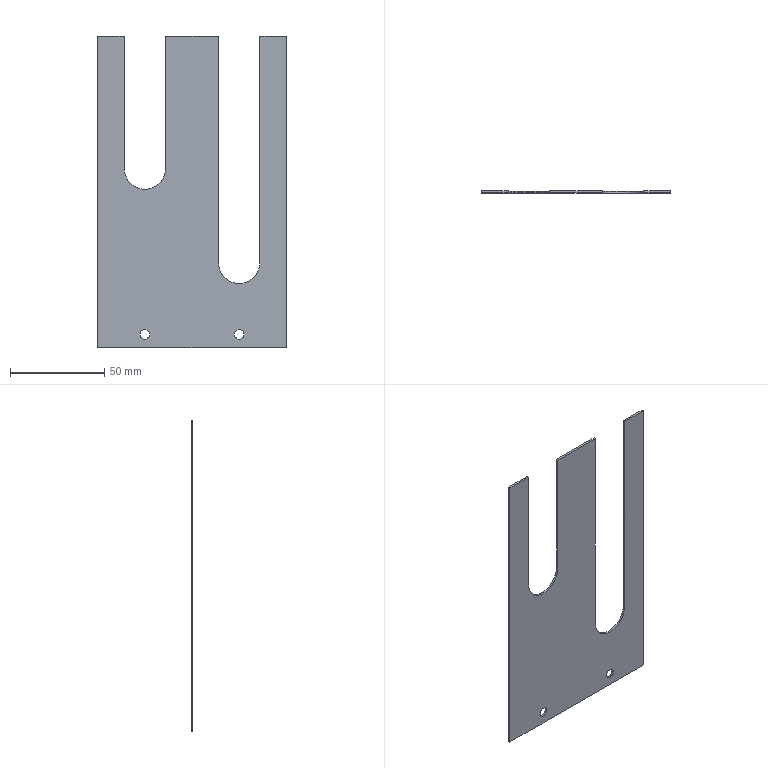Part | SolidWorks | features Extrusion 1, ICE 1 | 1 solid | 18 faces | box 100 x 1 x 165 mm | volume 11901 mm3 | plane 12 | cylinder 6 | commonest cylinder face diameters 5 x4 22 x2
STEP:
#1=CARTESIAN_POINT('',(-25.,0.,-78.));
#2=VERTEX_POINT('',#1);
#3=CARTESIAN_POINT('',(-25.,0.,-73.));
#4=VERTEX_POINT('',#3);
#5=CARTESIAN_POINT('',(-25.,0.,-75.5));
#6=DIRECTION('',(0.,1.,0.));
#7=DIRECTION('',(0.,0.,1.));
#8=AXIS2_PLACEMENT_3D('',#5,#6,#7);
#9=CIRCLE('',#8,2.5);
#10=EDGE_CURVE('',#2,#4,#9,.T.);
#11=ORIENTED_EDGE('',*,*,#10,.F.);
#12=CARTESIAN_POINT('',(-25.,1.,-78.));
#13=VERTEX_POINT('',#12);
#14=CARTESIAN_POINT('',(-25.,0.,-78.));
#15=DIRECTION('',(0.,1.,0.));
#16=VECTOR('',#15,1000.);
#17=LINE('',#14,#16);
#18=EDGE_CURVE('',#2,#13,#17,.T.);
#19=ORIENTED_EDGE('',*,*,#18,.T.);
#20=CARTESIAN_POINT('',(-25.,1.,-73.));
#21=VERTEX_POINT('',#20);
#22=CARTESIAN_POINT('',(-25.,1.,-75.5));
#23=DIRECTION('',(0.,1.,0.));
#24=DIRECTION('',(0.,0.,1.));
#25=AXIS2_PLACEMENT_3D('',#22,#23,#24);
#26=CIRCLE('',#25,2.5);
#27=EDGE_CURVE('',#13,#21,#26,.T.);
#28=ORIENTED_EDGE('',*,*,#27,.T.);
#29=CARTESIAN_POINT('',(-25.,0.,-73.));
#30=DIRECTION('',(0.,1.,0.));
#31=VECTOR('',#30,1000.);
#32=LINE('',#29,#31);
#33=EDGE_CURVE('',#4,#21,#32,.T.);
#34=ORIENTED_EDGE('',*,*,#33,.F.);
#35=EDGE_LOOP('',(#11,#19,#28,#34));
#36=FACE_OUTER_BOUND('',#35,.T.);
#37=CARTESIAN_POINT('',(-25.,0.,-75.5));
#38=DIRECTION('',(0.,1.,0.));
#39=DIRECTION('',(0.,0.,1.));
#40=AXIS2_PLACEMENT_3D('',#37,#38,#39);
#41=CYLINDRICAL_SURFACE('',#40,2.5);
#42=ADVANCED_FACE('',(#36),#41,.F.);
#43=CARTESIAN_POINT('',(25.,0.,-78.));
#44=VERTEX_POINT('',#43);
#45=CARTESIAN_POINT('',(25.,0.,-73.));
#46=VERTEX_POINT('',#45);
#47=CARTESIAN_POINT('',(25.,0.,-75.5));
#48=DIRECTION('',(0.,1.,0.));
#49=DIRECTION('',(0.,0.,1.));
#50=AXIS2_PLACEMENT_3D('',#47,#48,#49);
#51=CIRCLE('',#50,2.5);
#52=EDGE_CURVE('',#44,#46,#51,.T.);
#53=ORIENTED_EDGE('',*,*,#52,.F.);
#54=CARTESIAN_POINT('',(25.,1.,-78.));
#55=VERTEX_POINT('',#54);
#56=CARTESIAN_POINT('',(25.,0.,-78.));
#57=DIRECTION('',(0.,1.,0.));
#58=VECTOR('',#57,1000.);
#59=LINE('',#56,#58);
#60=EDGE_CURVE('',#44,#55,#59,.T.);
#61=ORIENTED_EDGE('',*,*,#60,.T.);
#62=CARTESIAN_POINT('',(25.,1.,-73.));
#63=VERTEX_POINT('',#62);
#64=CARTESIAN_POINT('',(25.,1.,-75.5));
#65=DIRECTION('',(0.,1.,0.));
#66=DIRECTION('',(0.,0.,1.));
#67=AXIS2_PLACEMENT_3D('',#64,#65,#66);
#68=CIRCLE('',#67,2.5);
#69=EDGE_CURVE('',#55,#63,#68,.T.);
#70=ORIENTED_EDGE('',*,*,#69,.T.);
#71=CARTESIAN_POINT('',(25.,0.,-73.));
#72=DIRECTION('',(0.,1.,0.));
#73=VECTOR('',#72,1000.);
#74=LINE('',#71,#73);
#75=EDGE_CURVE('',#46,#63,#74,.T.);
#76=ORIENTED_EDGE('',*,*,#75,.F.);
#77=EDGE_LOOP('',(#53,#61,#70,#76));
#78=FACE_OUTER_BOUND('',#77,.T.);
#79=CARTESIAN_POINT('',(25.,0.,-75.5));
#80=DIRECTION('',(0.,1.,0.));
#81=DIRECTION('',(0.,0.,1.));
#82=AXIS2_PLACEMENT_3D('',#79,#80,#81);
#83=CYLINDRICAL_SURFACE('',#82,2.5);
#84=ADVANCED_FACE('',(#78),#83,.F.);
#85=CARTESIAN_POINT('',(-14.,0.,82.5));
#86=VERTEX_POINT('',#85);
#87=CARTESIAN_POINT('',(14.,0.,82.5));
#88=VERTEX_POINT('',#87);
#89=CARTESIAN_POINT('',(-50.,0.,82.5));
#90=DIRECTION('',(1.,0.,0.));
#91=VECTOR('',#90,1000.);
#92=LINE('',#89,#91);
#93=EDGE_CURVE('',#86,#88,#92,.T.);
#94=ORIENTED_EDGE('',*,*,#93,.T.);
#95=CARTESIAN_POINT('',(14.,1.,82.5));
#96=VERTEX_POINT('',#95);
#97=CARTESIAN_POINT('',(14.,0.,82.5));
#98=DIRECTION('',(0.,1.,0.));
#99=VECTOR('',#98,1000.);
#100=LINE('',#97,#99);
#101=EDGE_CURVE('',#88,#96,#100,.T.);
#102=ORIENTED_EDGE('',*,*,#101,.T.);
#103=CARTESIAN_POINT('',(-14.,1.,82.5));
#104=VERTEX_POINT('',#103);
#105=CARTESIAN_POINT('',(-50.,1.,82.5));
#106=DIRECTION('',(1.,0.,0.));
#107=VECTOR('',#106,1000.);
#108=LINE('',#105,#107);
#109=EDGE_CURVE('',#104,#96,#108,.T.);
#110=ORIENTED_EDGE('',*,*,#109,.F.);
#111=CARTESIAN_POINT('',(-14.,0.,82.5));
#112=DIRECTION('',(0.,1.,0.));
#113=VECTOR('',#112,1000.);
#114=LINE('',#111,#113);
#115=EDGE_CURVE('',#86,#104,#114,.T.);
#116=ORIENTED_EDGE('',*,*,#115,.F.);
#117=EDGE_LOOP('',(#94,#102,#110,#116));
#118=FACE_OUTER_BOUND('',#117,.T.);
#119=CARTESIAN_POINT('',(-50.,1.,82.5));
#120=DIRECTION('',(0.,0.,-1.));
#121=DIRECTION('',(-1.,0.,0.));
#122=AXIS2_PLACEMENT_3D('',#119,#120,#121);
#123=PLANE('',#122);
#124=ADVANCED_FACE('',(#118),#123,.F.);
#125=CARTESIAN_POINT('',(-50.,0.,82.5));
#126=VERTEX_POINT('',#125);
#127=CARTESIAN_POINT('',(-36.,0.,82.5));
#128=VERTEX_POINT('',#127);
#129=CARTESIAN_POINT('',(-50.,0.,82.5));
#130=DIRECTION('',(1.,0.,0.));
#131=VECTOR('',#130,1000.);
#132=LINE('',#129,#131);
#133=EDGE_CURVE('',#126,#128,#132,.T.);
#134=ORIENTED_EDGE('',*,*,#133,.T.);
#135=CARTESIAN_POINT('',(-36.,1.,82.5));
#136=VERTEX_POINT('',#135);
#137=CARTESIAN_POINT('',(-36.,0.,82.5));
#138=DIRECTION('',(0.,1.,0.));
#139=VECTOR('',#138,1000.);
#140=LINE('',#137,#139);
#141=EDGE_CURVE('',#128,#136,#140,.T.);
#142=ORIENTED_EDGE('',*,*,#141,.T.);
#143=CARTESIAN_POINT('',(-50.,1.,82.5));
#144=VERTEX_POINT('',#143);
#145=CARTESIAN_POINT('',(-50.,1.,82.5));
#146=DIRECTION('',(1.,0.,0.));
#147=VECTOR('',#146,1000.);
#148=LINE('',#145,#147);
#149=EDGE_CURVE('',#144,#136,#148,.T.);
#150=ORIENTED_EDGE('',*,*,#149,.F.);
#151=CARTESIAN_POINT('',(-50.,1.,82.5));
#152=DIRECTION('',(0.,-1.,0.));
#153=VECTOR('',#152,1000.);
#154=LINE('',#151,#153);
#155=EDGE_CURVE('',#144,#126,#154,.T.);
#156=ORIENTED_EDGE('',*,*,#155,.T.);
#157=EDGE_LOOP('',(#134,#142,#150,#156));
#158=FACE_OUTER_BOUND('',#157,.T.);
#159=CARTESIAN_POINT('',(-50.,1.,82.5));
#160=DIRECTION('',(0.,0.,-1.));
#161=DIRECTION('',(-1.,0.,0.));
#162=AXIS2_PLACEMENT_3D('',#159,#160,#161);
#163=PLANE('',#162);
#164=ADVANCED_FACE('',(#158),#163,.F.);
#165=CARTESIAN_POINT('',(50.,0.,82.5));
#166=VERTEX_POINT('',#165);
#167=CARTESIAN_POINT('',(50.,0.,-82.5));
#168=VERTEX_POINT('',#167);
#169=CARTESIAN_POINT('',(50.,0.,82.5));
#170=DIRECTION('',(0.,0.,-1.));
#171=VECTOR('',#170,1000.);
#172=LINE('',#169,#171);
#173=EDGE_CURVE('',#166,#168,#172,.T.);
#174=ORIENTED_EDGE('',*,*,#173,.T.);
#175=CARTESIAN_POINT('',(50.,1.,-82.5));
#176=VERTEX_POINT('',#175);
#177=CARTESIAN_POINT('',(50.,1.,-82.5));
#178=DIRECTION('',(0.,-1.,0.));
#179=VECTOR('',#178,1000.);
#180=LINE('',#177,#179);
#181=EDGE_CURVE('',#176,#168,#180,.T.);
#182=ORIENTED_EDGE('',*,*,#181,.F.);
#183=CARTESIAN_POINT('',(50.,1.,82.5));
#184=VERTEX_POINT('',#183);
#185=CARTESIAN_POINT('',(50.,1.,82.5));
#186=DIRECTION('',(0.,0.,-1.));
#187=VECTOR('',#186,1000.);
#188=LINE('',#185,#187);
#189=EDGE_CURVE('',#184,#176,#188,.T.);
#190=ORIENTED_EDGE('',*,*,#189,.F.);
#191=CARTESIAN_POINT('',(50.,1.,82.5));
#192=DIRECTION('',(0.,-1.,0.));
#193=VECTOR('',#192,1000.);
#194=LINE('',#191,#193);
#195=EDGE_CURVE('',#184,#166,#194,.T.);
#196=ORIENTED_EDGE('',*,*,#195,.T.);
#197=EDGE_LOOP('',(#174,#182,#190,#196));
#198=FACE_OUTER_BOUND('',#197,.T.);
#199=CARTESIAN_POINT('',(50.,1.,82.5));
#200=DIRECTION('',(-1.,0.,0.));
#201=DIRECTION('',(0.,0.,1.));
#202=AXIS2_PLACEMENT_3D('',#199,#200,#201);
#203=PLANE('',#202);
#204=ADVANCED_FACE('',(#198),#203,.F.);
#205=CARTESIAN_POINT('',(-50.,0.,-82.5));
#206=VERTEX_POINT('',#205);
#207=CARTESIAN_POINT('',(-50.,0.,-82.5));
#208=DIRECTION('',(-1.,0.,0.));
#209=VECTOR('',#208,1000.);
#210=LINE('',#207,#209);
#211=EDGE_CURVE('',#168,#206,#210,.T.);
#212=ORIENTED_EDGE('',*,*,#211,.T.);
#213=CARTESIAN_POINT('',(-50.,1.,-82.5));
#214=VERTEX_POINT('',#213);
#215=CARTESIAN_POINT('',(-50.,1.,-82.5));
#216=DIRECTION('',(0.,-1.,0.));
#217=VECTOR('',#216,1000.);
#218=LINE('',#215,#217);
#219=EDGE_CURVE('',#214,#206,#218,.T.);
#220=ORIENTED_EDGE('',*,*,#219,.F.);
#221=CARTESIAN_POINT('',(-50.,1.,-82.5));
#222=DIRECTION('',(-1.,0.,0.));
#223=VECTOR('',#222,1000.);
#224=LINE('',#221,#223);
#225=EDGE_CURVE('',#176,#214,#224,.T.);
#226=ORIENTED_EDGE('',*,*,#225,.F.);
#227=ORIENTED_EDGE('',*,*,#181,.T.);
#228=EDGE_LOOP('',(#212,#220,#226,#227));
#229=FACE_OUTER_BOUND('',#228,.T.);
#230=CARTESIAN_POINT('',(-50.,1.,-82.5));
#231=DIRECTION('',(0.,0.,1.));
#232=DIRECTION('',(1.,0.,0.));
#233=AXIS2_PLACEMENT_3D('',#230,#231,#232);
#234=PLANE('',#233);
#235=ADVANCED_FACE('',(#229),#234,.F.);
#236=CARTESIAN_POINT('',(-50.,0.,82.5));
#237=DIRECTION('',(0.,0.,1.));
#238=VECTOR('',#237,1000.);
#239=LINE('',#236,#238);
#240=EDGE_CURVE('',#206,#126,#239,.T.);
#241=ORIENTED_EDGE('',*,*,#240,.T.);
#242=ORIENTED_EDGE('',*,*,#155,.F.);
#243=CARTESIAN_POINT('',(-50.,1.,82.5));
#244=DIRECTION('',(0.,0.,1.));
#245=VECTOR('',#244,1000.);
#246=LINE('',#243,#245);
#247=EDGE_CURVE('',#214,#144,#246,.T.);
#248=ORIENTED_EDGE('',*,*,#247,.F.);
#249=ORIENTED_EDGE('',*,*,#219,.T.);
#250=EDGE_LOOP('',(#241,#242,#248,#249));
#251=FACE_OUTER_BOUND('',#250,.T.);
#252=CARTESIAN_POINT('',(-50.,1.,82.5));
#253=DIRECTION('',(1.,0.,0.));
#254=DIRECTION('',(0.,0.,-1.));
#255=AXIS2_PLACEMENT_3D('',#252,#253,#254);
#256=PLANE('',#255);
#257=ADVANCED_FACE('',(#251),#256,.F.);
#258=CARTESIAN_POINT('',(36.,1.,82.5));
#259=VERTEX_POINT('',#258);
#260=CARTESIAN_POINT('',(-50.,1.,82.5));
#261=DIRECTION('',(1.,0.,0.));
#262=VECTOR('',#261,1000.);
#263=LINE('',#260,#262);
#264=EDGE_CURVE('',#259,#184,#263,.T.);
#265=ORIENTED_EDGE('',*,*,#264,.F.);
#266=CARTESIAN_POINT('',(36.,0.,82.5));
#267=VERTEX_POINT('',#266);
#268=CARTESIAN_POINT('',(36.,0.,82.5));
#269=DIRECTION('',(0.,1.,0.));
#270=VECTOR('',#269,1000.);
#271=LINE('',#268,#270);
#272=EDGE_CURVE('',#267,#259,#271,.T.);
#273=ORIENTED_EDGE('',*,*,#272,.F.);
#274=CARTESIAN_POINT('',(-50.,0.,82.5));
#275=DIRECTION('',(1.,0.,0.));
#276=VECTOR('',#275,1000.);
#277=LINE('',#274,#276);
#278=EDGE_CURVE('',#267,#166,#277,.T.);
#279=ORIENTED_EDGE('',*,*,#278,.T.);
#280=ORIENTED_EDGE('',*,*,#195,.F.);
#281=EDGE_LOOP('',(#265,#273,#279,#280));
#282=FACE_OUTER_BOUND('',#281,.T.);
#283=CARTESIAN_POINT('',(-50.,1.,82.5));
#284=DIRECTION('',(0.,0.,-1.));
#285=DIRECTION('',(-1.,0.,0.));
#286=AXIS2_PLACEMENT_3D('',#283,#284,#285);
#287=PLANE('',#286);
#288=ADVANCED_FACE('',(#282),#287,.F.);
#289=CARTESIAN_POINT('',(-25.,1.,-75.5));
#290=DIRECTION('',(0.,1.,0.));
#291=DIRECTION('',(0.,0.,1.));
#292=AXIS2_PLACEMENT_3D('',#289,#290,#291);
#293=CIRCLE('',#292,2.5);
#294=EDGE_CURVE('',#21,#13,#293,.T.);
#295=ORIENTED_EDGE('',*,*,#294,.F.);
#296=ORIENTED_EDGE('',*,*,#27,.F.);
#297=EDGE_LOOP('',(#295,#296));
#298=FACE_BOUND('',#297,.T.);
#299=CARTESIAN_POINT('',(25.,1.,-75.5));
#300=DIRECTION('',(0.,1.,0.));
#301=DIRECTION('',(0.,0.,1.));
#302=AXIS2_PLACEMENT_3D('',#299,#300,#301);
#303=CIRCLE('',#302,2.5);
#304=EDGE_CURVE('',#63,#55,#303,.T.);
#305=ORIENTED_EDGE('',*,*,#304,.F.);
#306=ORIENTED_EDGE('',*,*,#69,.F.);
#307=EDGE_LOOP('',(#305,#306));
#308=FACE_BOUND('',#307,.T.);
#309=ORIENTED_EDGE('',*,*,#109,.T.);
#310=CARTESIAN_POINT('',(14.,1.,-37.5));
#311=VERTEX_POINT('',#310);
#312=CARTESIAN_POINT('',(14.,1.,82.5));
#313=DIRECTION('',(0.,0.,1.));
#314=VECTOR('',#313,1000.);
#315=LINE('',#312,#314);
#316=EDGE_CURVE('',#311,#96,#315,.T.);
#317=ORIENTED_EDGE('',*,*,#316,.F.);
#318=CARTESIAN_POINT('',(36.,1.,-37.5));
#319=VERTEX_POINT('',#318);
#320=CARTESIAN_POINT('',(25.,1.,-37.5));
#321=DIRECTION('',(0.,1.,0.));
#322=DIRECTION('',(0.,0.,1.));
#323=AXIS2_PLACEMENT_3D('',#320,#321,#322);
#324=CIRCLE('',#323,11.);
#325=EDGE_CURVE('',#319,#311,#324,.T.);
#326=ORIENTED_EDGE('',*,*,#325,.F.);
#327=CARTESIAN_POINT('',(36.,1.,82.5));
#328=DIRECTION('',(0.,0.,-1.));
#329=VECTOR('',#328,1000.);
#330=LINE('',#327,#329);
#331=EDGE_CURVE('',#259,#319,#330,.T.);
#332=ORIENTED_EDGE('',*,*,#331,.F.);
#333=ORIENTED_EDGE('',*,*,#264,.T.);
#334=ORIENTED_EDGE('',*,*,#189,.T.);
#335=ORIENTED_EDGE('',*,*,#225,.T.);
#336=ORIENTED_EDGE('',*,*,#247,.T.);
#337=ORIENTED_EDGE('',*,*,#149,.T.);
#338=CARTESIAN_POINT('',(-36.,1.,12.5));
#339=VERTEX_POINT('',#338);
#340=CARTESIAN_POINT('',(-36.,1.,82.5));
#341=DIRECTION('',(0.,0.,1.));
#342=VECTOR('',#341,1000.);
#343=LINE('',#340,#342);
#344=EDGE_CURVE('',#339,#136,#343,.T.);
#345=ORIENTED_EDGE('',*,*,#344,.F.);
#346=CARTESIAN_POINT('',(-14.,1.,12.5));
#347=VERTEX_POINT('',#346);
#348=CARTESIAN_POINT('',(-25.,1.,12.5));
#349=DIRECTION('',(0.,1.,0.));
#350=DIRECTION('',(0.,0.,1.));
#351=AXIS2_PLACEMENT_3D('',#348,#349,#350);
#352=CIRCLE('',#351,11.);
#353=EDGE_CURVE('',#347,#339,#352,.T.);
#354=ORIENTED_EDGE('',*,*,#353,.F.);
#355=CARTESIAN_POINT('',(-14.,1.,82.5));
#356=DIRECTION('',(0.,0.,-1.));
#357=VECTOR('',#356,1000.);
#358=LINE('',#355,#357);
#359=EDGE_CURVE('',#104,#347,#358,.T.);
#360=ORIENTED_EDGE('',*,*,#359,.F.);
#361=EDGE_LOOP('',(#309,#317,#326,#332,#333,#334,#335,#336,#337,#345,#354,#360));
#362=FACE_OUTER_BOUND('',#361,.T.);
#363=CARTESIAN_POINT('',(0.,1.,0.));
#364=DIRECTION('',(0.,-1.,0.));
#365=DIRECTION('',(0.,0.,-1.));
#366=AXIS2_PLACEMENT_3D('',#363,#364,#365);
#367=PLANE('',#366);
#368=ADVANCED_FACE('',(#298,#308,#362),#367,.F.);
#369=CARTESIAN_POINT('',(14.,0.,-37.5));
#370=VERTEX_POINT('',#369);
#371=CARTESIAN_POINT('',(14.,0.,82.5));
#372=DIRECTION('',(0.,0.,1.));
#373=VECTOR('',#372,1000.);
#374=LINE('',#371,#373);
#375=EDGE_CURVE('',#370,#88,#374,.T.);
#376=ORIENTED_EDGE('',*,*,#375,.T.);
#377=ORIENTED_EDGE('',*,*,#93,.F.);
#378=CARTESIAN_POINT('',(-14.,0.,12.5));
#379=VERTEX_POINT('',#378);
#380=CARTESIAN_POINT('',(-14.,0.,82.5));
#381=DIRECTION('',(0.,0.,-1.));
#382=VECTOR('',#381,1000.);
#383=LINE('',#380,#382);
#384=EDGE_CURVE('',#86,#379,#383,.T.);
#385=ORIENTED_EDGE('',*,*,#384,.T.);
#386=CARTESIAN_POINT('',(-36.,0.,12.5));
#387=VERTEX_POINT('',#386);
#388=CARTESIAN_POINT('',(-25.,0.,12.5));
#389=DIRECTION('',(0.,1.,0.));
#390=DIRECTION('',(0.,0.,1.));
#391=AXIS2_PLACEMENT_3D('',#388,#389,#390);
#392=CIRCLE('',#391,11.);
#393=EDGE_CURVE('',#379,#387,#392,.T.);
#394=ORIENTED_EDGE('',*,*,#393,.T.);
#395=CARTESIAN_POINT('',(-36.,0.,82.5));
#396=DIRECTION('',(0.,0.,1.));
#397=VECTOR('',#396,1000.);
#398=LINE('',#395,#397);
#399=EDGE_CURVE('',#387,#128,#398,.T.);
#400=ORIENTED_EDGE('',*,*,#399,.T.);
#401=ORIENTED_EDGE('',*,*,#133,.F.);
#402=ORIENTED_EDGE('',*,*,#240,.F.);
#403=ORIENTED_EDGE('',*,*,#211,.F.);
#404=ORIENTED_EDGE('',*,*,#173,.F.);
#405=ORIENTED_EDGE('',*,*,#278,.F.);
#406=CARTESIAN_POINT('',(36.,0.,-37.5));
#407=VERTEX_POINT('',#406);
#408=CARTESIAN_POINT('',(36.,0.,82.5));
#409=DIRECTION('',(0.,0.,-1.));
#410=VECTOR('',#409,1000.);
#411=LINE('',#408,#410);
#412=EDGE_CURVE('',#267,#407,#411,.T.);
#413=ORIENTED_EDGE('',*,*,#412,.T.);
#414=CARTESIAN_POINT('',(25.,0.,-37.5));
#415=DIRECTION('',(0.,1.,0.));
#416=DIRECTION('',(0.,0.,1.));
#417=AXIS2_PLACEMENT_3D('',#414,#415,#416);
#418=CIRCLE('',#417,11.);
#419=EDGE_CURVE('',#407,#370,#418,.T.);
#420=ORIENTED_EDGE('',*,*,#419,.T.);
#421=EDGE_LOOP('',(#376,#377,#385,#394,#400,#401,#402,#403,#404,#405,#413,#420));
#422=FACE_OUTER_BOUND('',#421,.T.);
#423=CARTESIAN_POINT('',(-25.,0.,-75.5));
#424=DIRECTION('',(0.,1.,0.));
#425=DIRECTION('',(0.,0.,1.));
#426=AXIS2_PLACEMENT_3D('',#423,#424,#425);
#427=CIRCLE('',#426,2.5);
#428=EDGE_CURVE('',#4,#2,#427,.T.);
#429=ORIENTED_EDGE('',*,*,#428,.T.);
#430=ORIENTED_EDGE('',*,*,#10,.T.);
#431=EDGE_LOOP('',(#429,#430));
#432=FACE_BOUND('',#431,.T.);
#433=CARTESIAN_POINT('',(25.,0.,-75.5));
#434=DIRECTION('',(0.,1.,0.));
#435=DIRECTION('',(0.,0.,1.));
#436=AXIS2_PLACEMENT_3D('',#433,#434,#435);
#437=CIRCLE('',#436,2.5);
#438=EDGE_CURVE('',#46,#44,#437,.T.);
#439=ORIENTED_EDGE('',*,*,#438,.T.);
#440=ORIENTED_EDGE('',*,*,#52,.T.);
#441=EDGE_LOOP('',(#439,#440));
#442=FACE_BOUND('',#441,.T.);
#443=CARTESIAN_POINT('',(0.,0.,0.));
#444=DIRECTION('',(0.,-1.,0.));
#445=DIRECTION('',(0.,0.,-1.));
#446=AXIS2_PLACEMENT_3D('',#443,#444,#445);
#447=PLANE('',#446);
#448=ADVANCED_FACE('',(#422,#432,#442),#447,.T.);
#449=ORIENTED_EDGE('',*,*,#344,.T.);
#450=ORIENTED_EDGE('',*,*,#141,.F.);
#451=ORIENTED_EDGE('',*,*,#399,.F.);
#452=CARTESIAN_POINT('',(-36.,0.,12.5));
#453=DIRECTION('',(0.,1.,0.));
#454=VECTOR('',#453,1000.);
#455=LINE('',#452,#454);
#456=EDGE_CURVE('',#387,#339,#455,.T.);
#457=ORIENTED_EDGE('',*,*,#456,.T.);
#458=EDGE_LOOP('',(#449,#450,#451,#457));
#459=FACE_OUTER_BOUND('',#458,.T.);
#460=CARTESIAN_POINT('',(-36.,0.,82.5));
#461=DIRECTION('',(-1.,0.,0.));
#462=DIRECTION('',(0.,0.,1.));
#463=AXIS2_PLACEMENT_3D('',#460,#461,#462);
#464=PLANE('',#463);
#465=ADVANCED_FACE('',(#459),#464,.F.);
#466=ORIENTED_EDGE('',*,*,#353,.T.);
#467=ORIENTED_EDGE('',*,*,#456,.F.);
#468=ORIENTED_EDGE('',*,*,#393,.F.);
#469=CARTESIAN_POINT('',(-14.,0.,12.5));
#470=DIRECTION('',(0.,1.,0.));
#471=VECTOR('',#470,1000.);
#472=LINE('',#469,#471);
#473=EDGE_CURVE('',#379,#347,#472,.T.);
#474=ORIENTED_EDGE('',*,*,#473,.T.);
#475=EDGE_LOOP('',(#466,#467,#468,#474));
#476=FACE_OUTER_BOUND('',#475,.T.);
#477=CARTESIAN_POINT('',(-25.,0.,12.5));
#478=DIRECTION('',(0.,1.,0.));
#479=DIRECTION('',(0.,0.,1.));
#480=AXIS2_PLACEMENT_3D('',#477,#478,#479);
#481=CYLINDRICAL_SURFACE('',#480,11.);
#482=ADVANCED_FACE('',(#476),#481,.F.);
#483=ORIENTED_EDGE('',*,*,#359,.T.);
#484=ORIENTED_EDGE('',*,*,#473,.F.);
#485=ORIENTED_EDGE('',*,*,#384,.F.);
#486=ORIENTED_EDGE('',*,*,#115,.T.);
#487=EDGE_LOOP('',(#483,#484,#485,#486));
#488=FACE_OUTER_BOUND('',#487,.T.);
#489=CARTESIAN_POINT('',(-14.,0.,82.5));
#490=DIRECTION('',(1.,0.,0.));
#491=DIRECTION('',(0.,0.,-1.));
#492=AXIS2_PLACEMENT_3D('',#489,#490,#491);
#493=PLANE('',#492);
#494=ADVANCED_FACE('',(#488),#493,.F.);
#495=ORIENTED_EDGE('',*,*,#60,.F.);
#496=ORIENTED_EDGE('',*,*,#438,.F.);
#497=ORIENTED_EDGE('',*,*,#75,.T.);
#498=ORIENTED_EDGE('',*,*,#304,.T.);
#499=EDGE_LOOP('',(#495,#496,#497,#498));
#500=FACE_OUTER_BOUND('',#499,.T.);
#501=CARTESIAN_POINT('',(25.,0.,-75.5));
#502=DIRECTION('',(0.,1.,0.));
#503=DIRECTION('',(0.,0.,1.));
#504=AXIS2_PLACEMENT_3D('',#501,#502,#503);
#505=CYLINDRICAL_SURFACE('',#504,2.5);
#506=ADVANCED_FACE('',(#500),#505,.F.);
#507=ORIENTED_EDGE('',*,*,#18,.F.);
#508=ORIENTED_EDGE('',*,*,#428,.F.);
#509=ORIENTED_EDGE('',*,*,#33,.T.);
#510=ORIENTED_EDGE('',*,*,#294,.T.);
#511=EDGE_LOOP('',(#507,#508,#509,#510));
#512=FACE_OUTER_BOUND('',#511,.T.);
#513=CARTESIAN_POINT('',(-25.,0.,-75.5));
#514=DIRECTION('',(0.,1.,0.));
#515=DIRECTION('',(0.,0.,1.));
#516=AXIS2_PLACEMENT_3D('',#513,#514,#515);
#517=CYLINDRICAL_SURFACE('',#516,2.5);
#518=ADVANCED_FACE('',(#512),#517,.F.);
#519=ORIENTED_EDGE('',*,*,#316,.T.);
#520=ORIENTED_EDGE('',*,*,#101,.F.);
#521=ORIENTED_EDGE('',*,*,#375,.F.);
#522=CARTESIAN_POINT('',(14.,0.,-37.5));
#523=DIRECTION('',(0.,1.,0.));
#524=VECTOR('',#523,1000.);
#525=LINE('',#522,#524);
#526=EDGE_CURVE('',#370,#311,#525,.T.);
#527=ORIENTED_EDGE('',*,*,#526,.T.);
#528=EDGE_LOOP('',(#519,#520,#521,#527));
#529=FACE_OUTER_BOUND('',#528,.T.);
#530=CARTESIAN_POINT('',(14.,0.,82.5));
#531=DIRECTION('',(-1.,0.,0.));
#532=DIRECTION('',(0.,0.,1.));
#533=AXIS2_PLACEMENT_3D('',#530,#531,#532);
#534=PLANE('',#533);
#535=ADVANCED_FACE('',(#529),#534,.F.);
#536=ORIENTED_EDGE('',*,*,#325,.T.);
#537=ORIENTED_EDGE('',*,*,#526,.F.);
#538=ORIENTED_EDGE('',*,*,#419,.F.);
#539=CARTESIAN_POINT('',(36.,0.,-37.5));
#540=DIRECTION('',(0.,1.,0.));
#541=VECTOR('',#540,1000.);
#542=LINE('',#539,#541);
#543=EDGE_CURVE('',#407,#319,#542,.T.);
#544=ORIENTED_EDGE('',*,*,#543,.T.);
#545=EDGE_LOOP('',(#536,#537,#538,#544));
#546=FACE_OUTER_BOUND('',#545,.T.);
#547=CARTESIAN_POINT('',(25.,0.,-37.5));
#548=DIRECTION('',(0.,1.,0.));
#549=DIRECTION('',(0.,0.,1.));
#550=AXIS2_PLACEMENT_3D('',#547,#548,#549);
#551=CYLINDRICAL_SURFACE('',#550,11.);
#552=ADVANCED_FACE('',(#546),#551,.F.);
#553=ORIENTED_EDGE('',*,*,#331,.T.);
#554=ORIENTED_EDGE('',*,*,#543,.F.);
#555=ORIENTED_EDGE('',*,*,#412,.F.);
#556=ORIENTED_EDGE('',*,*,#272,.T.);
#557=EDGE_LOOP('',(#553,#554,#555,#556));
#558=FACE_OUTER_BOUND('',#557,.T.);
#559=CARTESIAN_POINT('',(36.,0.,82.5));
#560=DIRECTION('',(1.,0.,0.));
#561=DIRECTION('',(0.,0.,-1.));
#562=AXIS2_PLACEMENT_3D('',#559,#560,#561);
#563=PLANE('',#562);
#564=ADVANCED_FACE('',(#558),#563,.F.);
#565=CLOSED_SHELL('',(#42,#84,#124,#164,#204,#235,#257,#288,#368,#448,#465,#482,#494,#506,#518,#535,#552,#564));
#566=MANIFOLD_SOLID_BREP('',#565);
#567=CARTESIAN_POINT('',(0.,0.,0.));
#568=DIRECTION('',(0.,0.,1.));
#569=DIRECTION('',(1.,0.,0.));
#570=AXIS2_PLACEMENT_3D('',#567,#568,#569);
#571=(LENGTH_UNIT()NAMED_UNIT(*)SI_UNIT(.MILLI.,.METRE.));
#572=UNCERTAINTY_MEASURE_WITH_UNIT(LENGTH_MEASURE(0.00001),#571,'','');
#573=(NAMED_UNIT(*)PLANE_ANGLE_UNIT()SI_UNIT($,.RADIAN.));
#574=(NAMED_UNIT(*)SI_UNIT($,.STERADIAN.)SOLID_ANGLE_UNIT());
#575=(GEOMETRIC_REPRESENTATION_CONTEXT(3)GLOBAL_UNCERTAINTY_ASSIGNED_CONTEXT((#572))GLOBAL_UNIT_ASSIGNED_CONTEXT((#571,#573,#574))REPRESENTATION_CONTEXT('',''));
#576=ADVANCED_BREP_SHAPE_REPRESENTATION('',(#566,#570),#575);